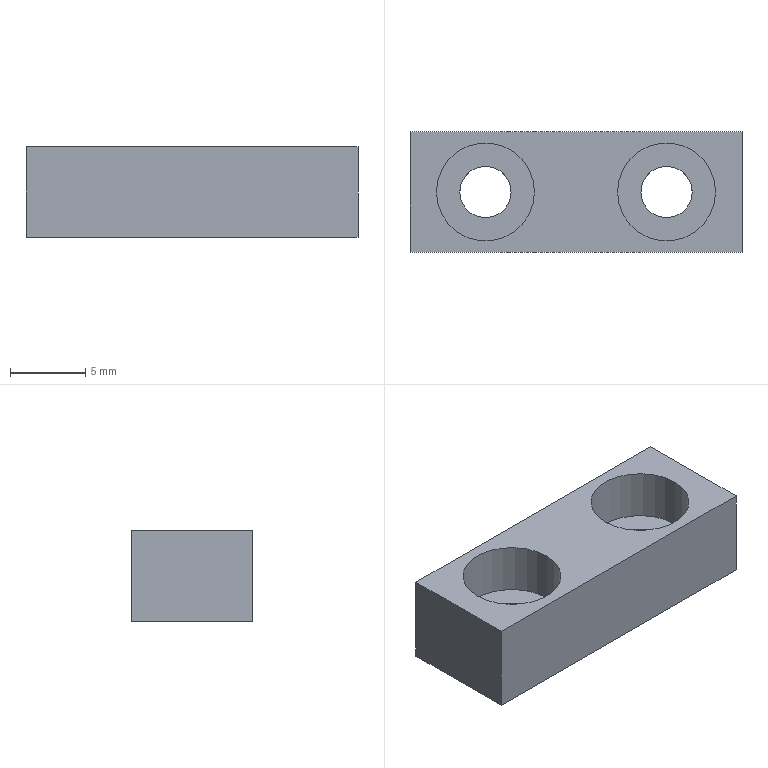Part | NX | 1 solid | 12 faces | box 22 x 8 x 6 mm | volume 783.143 mm3 | plane 8 | cylinder 4 | commonest cylinder face diameters 3.4 x2 6.5 x2
STEP:
#1=CARTESIAN_POINT('',(11.,-4.,0.));
#2=VERTEX_POINT('',#1);
#3=CARTESIAN_POINT('',(11.,4.,0.));
#4=VERTEX_POINT('',#3);
#5=CARTESIAN_POINT('',(11.,-4.,0.));
#6=DIRECTION('',(0.,1.,0.));
#7=VECTOR('',#6,1000.);
#8=LINE('',#5,#7);
#9=EDGE_CURVE('',#2,#4,#8,.T.);
#10=ORIENTED_EDGE('',*,*,#9,.T.);
#11=CARTESIAN_POINT('',(11.,4.,6.));
#12=VERTEX_POINT('',#11);
#13=CARTESIAN_POINT('',(11.,4.,6.));
#14=DIRECTION('',(0.,0.,-1.));
#15=VECTOR('',#14,1000.);
#16=LINE('',#13,#15);
#17=EDGE_CURVE('',#12,#4,#16,.T.);
#18=ORIENTED_EDGE('',*,*,#17,.F.);
#19=CARTESIAN_POINT('',(11.,-4.,6.));
#20=VERTEX_POINT('',#19);
#21=CARTESIAN_POINT('',(11.,-4.,6.));
#22=DIRECTION('',(0.,1.,0.));
#23=VECTOR('',#22,1000.);
#24=LINE('',#21,#23);
#25=EDGE_CURVE('',#20,#12,#24,.T.);
#26=ORIENTED_EDGE('',*,*,#25,.F.);
#27=CARTESIAN_POINT('',(11.,-4.,6.));
#28=DIRECTION('',(0.,0.,-1.));
#29=VECTOR('',#28,1000.);
#30=LINE('',#27,#29);
#31=EDGE_CURVE('',#20,#2,#30,.T.);
#32=ORIENTED_EDGE('',*,*,#31,.T.);
#33=EDGE_LOOP('',(#10,#18,#26,#32));
#34=FACE_BOUND('',#33,.T.);
#35=CARTESIAN_POINT('',(11.,-4.,6.));
#36=DIRECTION('',(-1.,0.,0.));
#37=DIRECTION('',(0.,0.,1.));
#38=AXIS2_PLACEMENT_3D('',#35,#36,#37);
#39=PLANE('',#38);
#40=ADVANCED_FACE('',(#34),#39,.F.);
#41=CARTESIAN_POINT('',(-11.,4.,0.));
#42=VERTEX_POINT('',#41);
#43=CARTESIAN_POINT('',(-11.,4.,0.));
#44=DIRECTION('',(-1.,0.,0.));
#45=VECTOR('',#44,1000.);
#46=LINE('',#43,#45);
#47=EDGE_CURVE('',#4,#42,#46,.T.);
#48=ORIENTED_EDGE('',*,*,#47,.T.);
#49=CARTESIAN_POINT('',(-11.,4.,6.));
#50=VERTEX_POINT('',#49);
#51=CARTESIAN_POINT('',(-11.,4.,6.));
#52=DIRECTION('',(0.,0.,-1.));
#53=VECTOR('',#52,1000.);
#54=LINE('',#51,#53);
#55=EDGE_CURVE('',#50,#42,#54,.T.);
#56=ORIENTED_EDGE('',*,*,#55,.F.);
#57=CARTESIAN_POINT('',(-11.,4.,6.));
#58=DIRECTION('',(-1.,0.,0.));
#59=VECTOR('',#58,1000.);
#60=LINE('',#57,#59);
#61=EDGE_CURVE('',#12,#50,#60,.T.);
#62=ORIENTED_EDGE('',*,*,#61,.F.);
#63=ORIENTED_EDGE('',*,*,#17,.T.);
#64=EDGE_LOOP('',(#48,#56,#62,#63));
#65=FACE_BOUND('',#64,.T.);
#66=CARTESIAN_POINT('',(-11.,4.,6.));
#67=DIRECTION('',(0.,-1.,0.));
#68=DIRECTION('',(0.,0.,-1.));
#69=AXIS2_PLACEMENT_3D('',#66,#67,#68);
#70=PLANE('',#69);
#71=ADVANCED_FACE('',(#65),#70,.F.);
#72=CARTESIAN_POINT('',(-11.,-4.,0.));
#73=VERTEX_POINT('',#72);
#74=CARTESIAN_POINT('',(-11.,-4.,0.));
#75=DIRECTION('',(0.,-1.,0.));
#76=VECTOR('',#75,1000.);
#77=LINE('',#74,#76);
#78=EDGE_CURVE('',#42,#73,#77,.T.);
#79=ORIENTED_EDGE('',*,*,#78,.T.);
#80=CARTESIAN_POINT('',(-11.,-4.,6.));
#81=VERTEX_POINT('',#80);
#82=CARTESIAN_POINT('',(-11.,-4.,6.));
#83=DIRECTION('',(0.,0.,-1.));
#84=VECTOR('',#83,1000.);
#85=LINE('',#82,#84);
#86=EDGE_CURVE('',#81,#73,#85,.T.);
#87=ORIENTED_EDGE('',*,*,#86,.F.);
#88=CARTESIAN_POINT('',(-11.,-4.,6.));
#89=DIRECTION('',(0.,-1.,0.));
#90=VECTOR('',#89,1000.);
#91=LINE('',#88,#90);
#92=EDGE_CURVE('',#50,#81,#91,.T.);
#93=ORIENTED_EDGE('',*,*,#92,.F.);
#94=ORIENTED_EDGE('',*,*,#55,.T.);
#95=EDGE_LOOP('',(#79,#87,#93,#94));
#96=FACE_BOUND('',#95,.T.);
#97=CARTESIAN_POINT('',(-11.,-4.,6.));
#98=DIRECTION('',(1.,0.,0.));
#99=DIRECTION('',(0.,0.,-1.));
#100=AXIS2_PLACEMENT_3D('',#97,#98,#99);
#101=PLANE('',#100);
#102=ADVANCED_FACE('',(#96),#101,.F.);
#103=CARTESIAN_POINT('',(-11.,-4.,0.));
#104=DIRECTION('',(1.,0.,0.));
#105=VECTOR('',#104,1000.);
#106=LINE('',#103,#105);
#107=EDGE_CURVE('',#73,#2,#106,.T.);
#108=ORIENTED_EDGE('',*,*,#107,.T.);
#109=ORIENTED_EDGE('',*,*,#31,.F.);
#110=CARTESIAN_POINT('',(-11.,-4.,6.));
#111=DIRECTION('',(1.,0.,0.));
#112=VECTOR('',#111,1000.);
#113=LINE('',#110,#112);
#114=EDGE_CURVE('',#81,#20,#113,.T.);
#115=ORIENTED_EDGE('',*,*,#114,.F.);
#116=ORIENTED_EDGE('',*,*,#86,.T.);
#117=EDGE_LOOP('',(#108,#109,#115,#116));
#118=FACE_BOUND('',#117,.T.);
#119=CARTESIAN_POINT('',(-11.,-4.,6.));
#120=DIRECTION('',(0.,1.,0.));
#121=DIRECTION('',(0.,0.,1.));
#122=AXIS2_PLACEMENT_3D('',#119,#120,#121);
#123=PLANE('',#122);
#124=ADVANCED_FACE('',(#118),#123,.F.);
#125=CARTESIAN_POINT('',(-2.75,0.,6.));
#126=VERTEX_POINT('',#125);
#127=CARTESIAN_POINT('',(-6.,0.,6.));
#128=DIRECTION('',(0.,0.,1.));
#129=DIRECTION('',(1.,0.,0.));
#130=AXIS2_PLACEMENT_3D('',#127,#128,#129);
#131=CIRCLE('',#130,3.25);
#132=EDGE_CURVE('',#126,#126,#131,.T.);
#133=ORIENTED_EDGE('',*,*,#132,.F.);
#134=EDGE_LOOP('',(#133));
#135=FACE_BOUND('',#134,.T.);
#136=CARTESIAN_POINT('',(9.25,0.,6.));
#137=VERTEX_POINT('',#136);
#138=CARTESIAN_POINT('',(6.,0.,6.));
#139=DIRECTION('',(0.,0.,1.));
#140=DIRECTION('',(1.,0.,0.));
#141=AXIS2_PLACEMENT_3D('',#138,#139,#140);
#142=CIRCLE('',#141,3.25);
#143=EDGE_CURVE('',#137,#137,#142,.T.);
#144=ORIENTED_EDGE('',*,*,#143,.F.);
#145=EDGE_LOOP('',(#144));
#146=FACE_BOUND('',#145,.T.);
#147=ORIENTED_EDGE('',*,*,#25,.T.);
#148=ORIENTED_EDGE('',*,*,#61,.T.);
#149=ORIENTED_EDGE('',*,*,#92,.T.);
#150=ORIENTED_EDGE('',*,*,#114,.T.);
#151=EDGE_LOOP('',(#147,#148,#149,#150));
#152=FACE_BOUND('',#151,.T.);
#153=CARTESIAN_POINT('',(0.,0.,6.));
#154=DIRECTION('',(0.,0.,-1.));
#155=DIRECTION('',(-1.,0.,0.));
#156=AXIS2_PLACEMENT_3D('',#153,#154,#155);
#157=PLANE('',#156);
#158=ADVANCED_FACE('',(#135,#146,#152),#157,.F.);
#159=CARTESIAN_POINT('',(-4.3,0.,0.));
#160=VERTEX_POINT('',#159);
#161=CARTESIAN_POINT('',(-6.,0.,0.));
#162=DIRECTION('',(0.,0.,1.));
#163=DIRECTION('',(1.,0.,0.));
#164=AXIS2_PLACEMENT_3D('',#161,#162,#163);
#165=CIRCLE('',#164,1.7);
#166=EDGE_CURVE('',#160,#160,#165,.T.);
#167=ORIENTED_EDGE('',*,*,#166,.T.);
#168=EDGE_LOOP('',(#167));
#169=FACE_BOUND('',#168,.T.);
#170=CARTESIAN_POINT('',(7.7,0.,0.));
#171=VERTEX_POINT('',#170);
#172=CARTESIAN_POINT('',(6.,0.,0.));
#173=DIRECTION('',(0.,0.,1.));
#174=DIRECTION('',(1.,0.,0.));
#175=AXIS2_PLACEMENT_3D('',#172,#173,#174);
#176=CIRCLE('',#175,1.7);
#177=EDGE_CURVE('',#171,#171,#176,.T.);
#178=ORIENTED_EDGE('',*,*,#177,.T.);
#179=EDGE_LOOP('',(#178));
#180=FACE_BOUND('',#179,.T.);
#181=ORIENTED_EDGE('',*,*,#9,.F.);
#182=ORIENTED_EDGE('',*,*,#107,.F.);
#183=ORIENTED_EDGE('',*,*,#78,.F.);
#184=ORIENTED_EDGE('',*,*,#47,.F.);
#185=EDGE_LOOP('',(#181,#182,#183,#184));
#186=FACE_BOUND('',#185,.T.);
#187=CARTESIAN_POINT('',(0.,0.,0.));
#188=DIRECTION('',(0.,0.,-1.));
#189=DIRECTION('',(-1.,0.,0.));
#190=AXIS2_PLACEMENT_3D('',#187,#188,#189);
#191=PLANE('',#190);
#192=ADVANCED_FACE('',(#169,#180,#186),#191,.T.);
#193=ORIENTED_EDGE('',*,*,#177,.F.);
#194=EDGE_LOOP('',(#193));
#195=FACE_BOUND('',#194,.T.);
#196=CARTESIAN_POINT('',(7.7,0.,2.6));
#197=VERTEX_POINT('',#196);
#198=CARTESIAN_POINT('',(6.,0.,2.6));
#199=DIRECTION('',(0.,0.,1.));
#200=DIRECTION('',(1.,0.,0.));
#201=AXIS2_PLACEMENT_3D('',#198,#199,#200);
#202=CIRCLE('',#201,1.7);
#203=EDGE_CURVE('',#197,#197,#202,.T.);
#204=ORIENTED_EDGE('',*,*,#203,.T.);
#205=EDGE_LOOP('',(#204));
#206=FACE_BOUND('',#205,.T.);
#207=CARTESIAN_POINT('',(6.,0.,6.));
#208=DIRECTION('',(0.,0.,1.));
#209=DIRECTION('',(1.,0.,0.));
#210=AXIS2_PLACEMENT_3D('',#207,#208,#209);
#211=CYLINDRICAL_SURFACE('',#210,1.7);
#212=ADVANCED_FACE('',(#195,#206),#211,.F.);
#213=ORIENTED_EDGE('',*,*,#203,.F.);
#214=EDGE_LOOP('',(#213));
#215=FACE_BOUND('',#214,.T.);
#216=CARTESIAN_POINT('',(9.25,0.,2.6));
#217=VERTEX_POINT('',#216);
#218=CARTESIAN_POINT('',(6.,0.,2.6));
#219=DIRECTION('',(0.,0.,1.));
#220=DIRECTION('',(1.,0.,0.));
#221=AXIS2_PLACEMENT_3D('',#218,#219,#220);
#222=CIRCLE('',#221,3.25);
#223=EDGE_CURVE('',#217,#217,#222,.T.);
#224=ORIENTED_EDGE('',*,*,#223,.T.);
#225=EDGE_LOOP('',(#224));
#226=FACE_BOUND('',#225,.T.);
#227=CARTESIAN_POINT('',(7.7,0.,2.6));
#228=DIRECTION('',(0.,0.,-1.));
#229=DIRECTION('',(-1.,0.,0.));
#230=AXIS2_PLACEMENT_3D('',#227,#228,#229);
#231=PLANE('',#230);
#232=ADVANCED_FACE('',(#215,#226),#231,.F.);
#233=ORIENTED_EDGE('',*,*,#223,.F.);
#234=EDGE_LOOP('',(#233));
#235=FACE_BOUND('',#234,.T.);
#236=ORIENTED_EDGE('',*,*,#143,.T.);
#237=EDGE_LOOP('',(#236));
#238=FACE_BOUND('',#237,.T.);
#239=CARTESIAN_POINT('',(6.,0.,6.));
#240=DIRECTION('',(0.,0.,1.));
#241=DIRECTION('',(1.,0.,0.));
#242=AXIS2_PLACEMENT_3D('',#239,#240,#241);
#243=CYLINDRICAL_SURFACE('',#242,3.25);
#244=ADVANCED_FACE('',(#235,#238),#243,.F.);
#245=ORIENTED_EDGE('',*,*,#166,.F.);
#246=EDGE_LOOP('',(#245));
#247=FACE_BOUND('',#246,.T.);
#248=CARTESIAN_POINT('',(-4.3,0.,2.6));
#249=VERTEX_POINT('',#248);
#250=CARTESIAN_POINT('',(-6.,0.,2.6));
#251=DIRECTION('',(0.,0.,1.));
#252=DIRECTION('',(1.,0.,0.));
#253=AXIS2_PLACEMENT_3D('',#250,#251,#252);
#254=CIRCLE('',#253,1.7);
#255=EDGE_CURVE('',#249,#249,#254,.T.);
#256=ORIENTED_EDGE('',*,*,#255,.T.);
#257=EDGE_LOOP('',(#256));
#258=FACE_BOUND('',#257,.T.);
#259=CARTESIAN_POINT('',(-6.,0.,6.));
#260=DIRECTION('',(0.,0.,1.));
#261=DIRECTION('',(1.,0.,0.));
#262=AXIS2_PLACEMENT_3D('',#259,#260,#261);
#263=CYLINDRICAL_SURFACE('',#262,1.7);
#264=ADVANCED_FACE('',(#247,#258),#263,.F.);
#265=ORIENTED_EDGE('',*,*,#255,.F.);
#266=EDGE_LOOP('',(#265));
#267=FACE_BOUND('',#266,.T.);
#268=CARTESIAN_POINT('',(-2.75,0.,2.6));
#269=VERTEX_POINT('',#268);
#270=CARTESIAN_POINT('',(-6.,0.,2.6));
#271=DIRECTION('',(0.,0.,1.));
#272=DIRECTION('',(1.,0.,0.));
#273=AXIS2_PLACEMENT_3D('',#270,#271,#272);
#274=CIRCLE('',#273,3.25);
#275=EDGE_CURVE('',#269,#269,#274,.T.);
#276=ORIENTED_EDGE('',*,*,#275,.T.);
#277=EDGE_LOOP('',(#276));
#278=FACE_BOUND('',#277,.T.);
#279=CARTESIAN_POINT('',(-4.3,0.,2.6));
#280=DIRECTION('',(0.,0.,-1.));
#281=DIRECTION('',(-1.,0.,0.));
#282=AXIS2_PLACEMENT_3D('',#279,#280,#281);
#283=PLANE('',#282);
#284=ADVANCED_FACE('',(#267,#278),#283,.F.);
#285=ORIENTED_EDGE('',*,*,#275,.F.);
#286=EDGE_LOOP('',(#285));
#287=FACE_BOUND('',#286,.T.);
#288=ORIENTED_EDGE('',*,*,#132,.T.);
#289=EDGE_LOOP('',(#288));
#290=FACE_BOUND('',#289,.T.);
#291=CARTESIAN_POINT('',(-6.,0.,6.));
#292=DIRECTION('',(0.,0.,1.));
#293=DIRECTION('',(1.,0.,0.));
#294=AXIS2_PLACEMENT_3D('',#291,#292,#293);
#295=CYLINDRICAL_SURFACE('',#294,3.25);
#296=ADVANCED_FACE('',(#287,#290),#295,.F.);
#297=CLOSED_SHELL('',(#40,#71,#102,#124,#158,#192,#212,#232,#244,#264,#284,#296));
#298=MANIFOLD_SOLID_BREP('',#297);
#299=(LENGTH_UNIT()NAMED_UNIT(*)SI_UNIT(.MILLI.,.METRE.));
#300=UNCERTAINTY_MEASURE_WITH_UNIT(LENGTH_MEASURE(0.00001),#299,'','');
#301=(NAMED_UNIT(*)PLANE_ANGLE_UNIT()SI_UNIT($,.RADIAN.));
#302=(NAMED_UNIT(*)SI_UNIT($,.STERADIAN.)SOLID_ANGLE_UNIT());
#303=(GEOMETRIC_REPRESENTATION_CONTEXT(3)GLOBAL_UNCERTAINTY_ASSIGNED_CONTEXT((#300))GLOBAL_UNIT_ASSIGNED_CONTEXT((#299,#301,#302))REPRESENTATION_CONTEXT('',''));
#304=ADVANCED_BREP_SHAPE_REPRESENTATION('',(#298),#303);